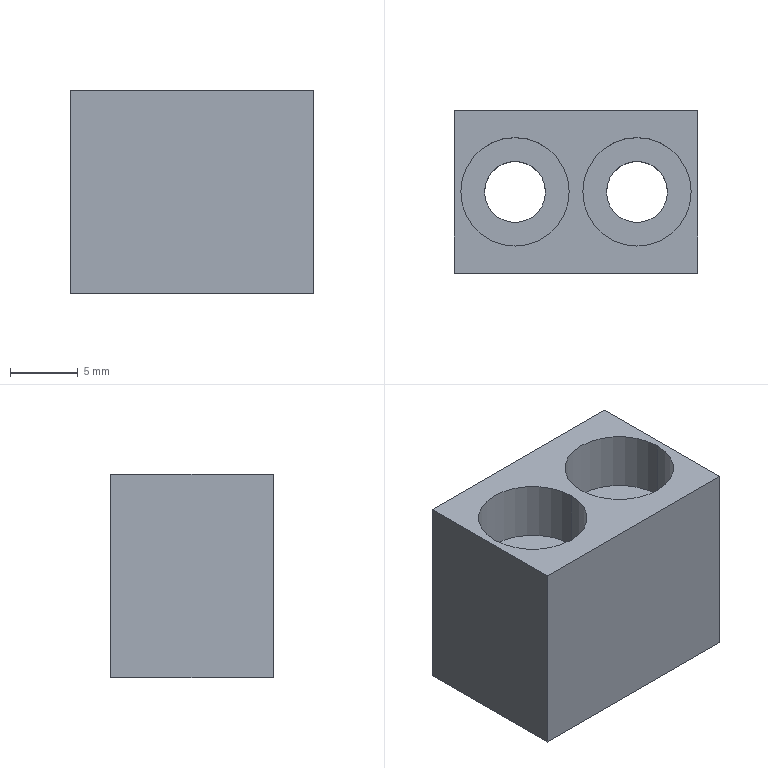Part | SolidWorks | features BaseBody 1 | 1 solid | 16 faces | box 18 x 12 x 15 mm | volume 2460 mm3 | cylinder 8 | plane 8 | commonest cylinder face diameters 4.5 x4 8 x4
STEP:
#1=CARTESIAN_POINT('',(-2.25,0.,0.));
#2=VERTEX_POINT('',#1);
#3=CARTESIAN_POINT('',(-6.75,0.,0.));
#4=VERTEX_POINT('',#3);
#5=CARTESIAN_POINT('',(-4.5,0.,0.));
#6=DIRECTION('',(0.,0.,-1.));
#7=DIRECTION('',(1.,0.,0.));
#8=AXIS2_PLACEMENT_3D('',#5,#6,#7);
#9=CIRCLE('',#8,2.25);
#10=EDGE_CURVE('',#2,#4,#9,.T.);
#11=ORIENTED_EDGE('',*,*,#10,.T.);
#12=CARTESIAN_POINT('',(-6.75,0.,10.6));
#13=VERTEX_POINT('',#12);
#14=CARTESIAN_POINT('',(-6.75,0.,15.));
#15=DIRECTION('',(0.,0.,1.));
#16=VECTOR('',#15,1000.);
#17=LINE('',#14,#16);
#18=EDGE_CURVE('',#4,#13,#17,.T.);
#19=ORIENTED_EDGE('',*,*,#18,.T.);
#20=CARTESIAN_POINT('',(-2.25,0.,10.6));
#21=VERTEX_POINT('',#20);
#22=CARTESIAN_POINT('',(-4.5,0.,10.6));
#23=DIRECTION('',(0.,0.,-1.));
#24=DIRECTION('',(1.,0.,0.));
#25=AXIS2_PLACEMENT_3D('',#22,#23,#24);
#26=CIRCLE('',#25,2.25);
#27=EDGE_CURVE('',#21,#13,#26,.T.);
#28=ORIENTED_EDGE('',*,*,#27,.F.);
#29=CARTESIAN_POINT('',(-2.25,0.,15.));
#30=DIRECTION('',(0.,0.,1.));
#31=VECTOR('',#30,1000.);
#32=LINE('',#29,#31);
#33=EDGE_CURVE('',#2,#21,#32,.T.);
#34=ORIENTED_EDGE('',*,*,#33,.F.);
#35=EDGE_LOOP('',(#11,#19,#28,#34));
#36=FACE_OUTER_BOUND('',#35,.T.);
#37=CARTESIAN_POINT('',(-4.5,0.,15.));
#38=DIRECTION('',(0.,0.,1.));
#39=DIRECTION('',(1.,0.,0.));
#40=AXIS2_PLACEMENT_3D('',#37,#38,#39);
#41=CYLINDRICAL_SURFACE('',#40,2.25);
#42=ADVANCED_FACE('',(#36),#41,.F.);
#43=CARTESIAN_POINT('',(6.75,0.,0.));
#44=VERTEX_POINT('',#43);
#45=CARTESIAN_POINT('',(2.25,0.,0.));
#46=VERTEX_POINT('',#45);
#47=CARTESIAN_POINT('',(4.5,0.,0.));
#48=DIRECTION('',(0.,0.,-1.));
#49=DIRECTION('',(1.,0.,0.));
#50=AXIS2_PLACEMENT_3D('',#47,#48,#49);
#51=CIRCLE('',#50,2.25);
#52=EDGE_CURVE('',#44,#46,#51,.T.);
#53=ORIENTED_EDGE('',*,*,#52,.T.);
#54=CARTESIAN_POINT('',(2.25,0.,10.6));
#55=VERTEX_POINT('',#54);
#56=CARTESIAN_POINT('',(2.25,0.,15.));
#57=DIRECTION('',(0.,0.,1.));
#58=VECTOR('',#57,1000.);
#59=LINE('',#56,#58);
#60=EDGE_CURVE('',#46,#55,#59,.T.);
#61=ORIENTED_EDGE('',*,*,#60,.T.);
#62=CARTESIAN_POINT('',(6.75,0.,10.6));
#63=VERTEX_POINT('',#62);
#64=CARTESIAN_POINT('',(4.5,0.,10.6));
#65=DIRECTION('',(0.,0.,-1.));
#66=DIRECTION('',(1.,0.,0.));
#67=AXIS2_PLACEMENT_3D('',#64,#65,#66);
#68=CIRCLE('',#67,2.25);
#69=EDGE_CURVE('',#63,#55,#68,.T.);
#70=ORIENTED_EDGE('',*,*,#69,.F.);
#71=CARTESIAN_POINT('',(6.75,0.,15.));
#72=DIRECTION('',(0.,0.,1.));
#73=VECTOR('',#72,1000.);
#74=LINE('',#71,#73);
#75=EDGE_CURVE('',#44,#63,#74,.T.);
#76=ORIENTED_EDGE('',*,*,#75,.F.);
#77=EDGE_LOOP('',(#53,#61,#70,#76));
#78=FACE_OUTER_BOUND('',#77,.T.);
#79=CARTESIAN_POINT('',(4.5,0.,15.));
#80=DIRECTION('',(0.,0.,1.));
#81=DIRECTION('',(1.,0.,0.));
#82=AXIS2_PLACEMENT_3D('',#79,#80,#81);
#83=CYLINDRICAL_SURFACE('',#82,2.25);
#84=ADVANCED_FACE('',(#78),#83,.F.);
#85=CARTESIAN_POINT('',(-8.5,0.,10.6));
#86=VERTEX_POINT('',#85);
#87=CARTESIAN_POINT('',(-0.5,0.,10.6));
#88=VERTEX_POINT('',#87);
#89=CARTESIAN_POINT('',(-4.5,0.,10.6));
#90=DIRECTION('',(0.,0.,1.));
#91=DIRECTION('',(1.,0.,0.));
#92=AXIS2_PLACEMENT_3D('',#89,#90,#91);
#93=CIRCLE('',#92,4.);
#94=EDGE_CURVE('',#86,#88,#93,.T.);
#95=ORIENTED_EDGE('',*,*,#94,.F.);
#96=CARTESIAN_POINT('',(-8.5,0.,15.));
#97=VERTEX_POINT('',#96);
#98=CARTESIAN_POINT('',(-8.5,0.,15.));
#99=DIRECTION('',(0.,0.,1.));
#100=VECTOR('',#99,1000.);
#101=LINE('',#98,#100);
#102=EDGE_CURVE('',#86,#97,#101,.T.);
#103=ORIENTED_EDGE('',*,*,#102,.T.);
#104=CARTESIAN_POINT('',(-0.5,0.,15.));
#105=VERTEX_POINT('',#104);
#106=CARTESIAN_POINT('',(-4.5,0.,15.));
#107=DIRECTION('',(0.,0.,-1.));
#108=DIRECTION('',(1.,0.,0.));
#109=AXIS2_PLACEMENT_3D('',#106,#107,#108);
#110=CIRCLE('',#109,4.);
#111=EDGE_CURVE('',#105,#97,#110,.T.);
#112=ORIENTED_EDGE('',*,*,#111,.F.);
#113=CARTESIAN_POINT('',(-0.5,0.,15.));
#114=DIRECTION('',(0.,0.,1.));
#115=VECTOR('',#114,1000.);
#116=LINE('',#113,#115);
#117=EDGE_CURVE('',#88,#105,#116,.T.);
#118=ORIENTED_EDGE('',*,*,#117,.F.);
#119=EDGE_LOOP('',(#95,#103,#112,#118));
#120=FACE_OUTER_BOUND('',#119,.T.);
#121=CARTESIAN_POINT('',(-4.5,0.,15.));
#122=DIRECTION('',(0.,0.,1.));
#123=DIRECTION('',(1.,0.,0.));
#124=AXIS2_PLACEMENT_3D('',#121,#122,#123);
#125=CYLINDRICAL_SURFACE('',#124,4.);
#126=ADVANCED_FACE('',(#120),#125,.F.);
#127=CARTESIAN_POINT('',(0.5,0.,10.6));
#128=VERTEX_POINT('',#127);
#129=CARTESIAN_POINT('',(8.5,0.,10.6));
#130=VERTEX_POINT('',#129);
#131=CARTESIAN_POINT('',(4.5,0.,10.6));
#132=DIRECTION('',(0.,0.,1.));
#133=DIRECTION('',(1.,0.,0.));
#134=AXIS2_PLACEMENT_3D('',#131,#132,#133);
#135=CIRCLE('',#134,4.);
#136=EDGE_CURVE('',#128,#130,#135,.T.);
#137=ORIENTED_EDGE('',*,*,#136,.F.);
#138=CARTESIAN_POINT('',(0.5,0.,15.));
#139=VERTEX_POINT('',#138);
#140=CARTESIAN_POINT('',(0.5,0.,15.));
#141=DIRECTION('',(0.,0.,1.));
#142=VECTOR('',#141,1000.);
#143=LINE('',#140,#142);
#144=EDGE_CURVE('',#128,#139,#143,.T.);
#145=ORIENTED_EDGE('',*,*,#144,.T.);
#146=CARTESIAN_POINT('',(8.5,0.,15.));
#147=VERTEX_POINT('',#146);
#148=CARTESIAN_POINT('',(4.5,0.,15.));
#149=DIRECTION('',(0.,0.,-1.));
#150=DIRECTION('',(1.,0.,0.));
#151=AXIS2_PLACEMENT_3D('',#148,#149,#150);
#152=CIRCLE('',#151,4.);
#153=EDGE_CURVE('',#147,#139,#152,.T.);
#154=ORIENTED_EDGE('',*,*,#153,.F.);
#155=CARTESIAN_POINT('',(8.5,0.,15.));
#156=DIRECTION('',(0.,0.,1.));
#157=VECTOR('',#156,1000.);
#158=LINE('',#155,#157);
#159=EDGE_CURVE('',#130,#147,#158,.T.);
#160=ORIENTED_EDGE('',*,*,#159,.F.);
#161=EDGE_LOOP('',(#137,#145,#154,#160));
#162=FACE_OUTER_BOUND('',#161,.T.);
#163=CARTESIAN_POINT('',(4.5,0.,15.));
#164=DIRECTION('',(0.,0.,1.));
#165=DIRECTION('',(1.,0.,0.));
#166=AXIS2_PLACEMENT_3D('',#163,#164,#165);
#167=CYLINDRICAL_SURFACE('',#166,4.);
#168=ADVANCED_FACE('',(#162),#167,.F.);
#169=CARTESIAN_POINT('',(-9.,6.,15.));
#170=VERTEX_POINT('',#169);
#171=CARTESIAN_POINT('',(-9.,6.,0.));
#172=VERTEX_POINT('',#171);
#173=CARTESIAN_POINT('',(-9.,6.,15.));
#174=DIRECTION('',(0.,0.,-1.));
#175=VECTOR('',#174,1000.);
#176=LINE('',#173,#175);
#177=EDGE_CURVE('',#170,#172,#176,.T.);
#178=ORIENTED_EDGE('',*,*,#177,.F.);
#179=CARTESIAN_POINT('',(9.,6.,15.));
#180=VERTEX_POINT('',#179);
#181=CARTESIAN_POINT('',(-9.,6.,15.));
#182=DIRECTION('',(-1.,0.,0.));
#183=VECTOR('',#182,1000.);
#184=LINE('',#181,#183);
#185=EDGE_CURVE('',#180,#170,#184,.T.);
#186=ORIENTED_EDGE('',*,*,#185,.F.);
#187=CARTESIAN_POINT('',(9.,6.,0.));
#188=VERTEX_POINT('',#187);
#189=CARTESIAN_POINT('',(9.,6.,15.));
#190=DIRECTION('',(0.,0.,1.));
#191=VECTOR('',#190,1000.);
#192=LINE('',#189,#191);
#193=EDGE_CURVE('',#188,#180,#192,.T.);
#194=ORIENTED_EDGE('',*,*,#193,.F.);
#195=CARTESIAN_POINT('',(-9.,6.,0.));
#196=DIRECTION('',(1.,0.,0.));
#197=VECTOR('',#196,1000.);
#198=LINE('',#195,#197);
#199=EDGE_CURVE('',#172,#188,#198,.T.);
#200=ORIENTED_EDGE('',*,*,#199,.F.);
#201=EDGE_LOOP('',(#178,#186,#194,#200));
#202=FACE_OUTER_BOUND('',#201,.T.);
#203=CARTESIAN_POINT('',(-9.,6.,15.));
#204=DIRECTION('',(0.,-1.,0.));
#205=DIRECTION('',(0.,0.,-1.));
#206=AXIS2_PLACEMENT_3D('',#203,#204,#205);
#207=PLANE('',#206);
#208=ADVANCED_FACE('',(#202),#207,.F.);
#209=CARTESIAN_POINT('',(-9.,-6.,0.));
#210=VERTEX_POINT('',#209);
#211=CARTESIAN_POINT('',(9.,-6.,0.));
#212=VERTEX_POINT('',#211);
#213=CARTESIAN_POINT('',(0.,-6.,0.));
#214=DIRECTION('',(1.,0.,0.));
#215=VECTOR('',#214,1000.);
#216=LINE('',#213,#215);
#217=EDGE_CURVE('',#210,#212,#216,.T.);
#218=ORIENTED_EDGE('',*,*,#217,.F.);
#219=CARTESIAN_POINT('',(-9.,0.,0.));
#220=DIRECTION('',(0.,-1.,0.));
#221=VECTOR('',#220,1000.);
#222=LINE('',#219,#221);
#223=EDGE_CURVE('',#172,#210,#222,.T.);
#224=ORIENTED_EDGE('',*,*,#223,.F.);
#225=ORIENTED_EDGE('',*,*,#199,.T.);
#226=CARTESIAN_POINT('',(9.,0.,0.));
#227=DIRECTION('',(0.,1.,0.));
#228=VECTOR('',#227,1000.);
#229=LINE('',#226,#228);
#230=EDGE_CURVE('',#212,#188,#229,.T.);
#231=ORIENTED_EDGE('',*,*,#230,.F.);
#232=EDGE_LOOP('',(#218,#224,#225,#231));
#233=FACE_OUTER_BOUND('',#232,.T.);
#234=ORIENTED_EDGE('',*,*,#10,.F.);
#235=CARTESIAN_POINT('',(-4.5,0.,0.));
#236=DIRECTION('',(0.,0.,-1.));
#237=DIRECTION('',(1.,0.,0.));
#238=AXIS2_PLACEMENT_3D('',#235,#236,#237);
#239=CIRCLE('',#238,2.25);
#240=EDGE_CURVE('',#4,#2,#239,.T.);
#241=ORIENTED_EDGE('',*,*,#240,.F.);
#242=EDGE_LOOP('',(#234,#241));
#243=FACE_BOUND('',#242,.T.);
#244=ORIENTED_EDGE('',*,*,#52,.F.);
#245=CARTESIAN_POINT('',(4.5,0.,0.));
#246=DIRECTION('',(0.,0.,-1.));
#247=DIRECTION('',(1.,0.,0.));
#248=AXIS2_PLACEMENT_3D('',#245,#246,#247);
#249=CIRCLE('',#248,2.25);
#250=EDGE_CURVE('',#46,#44,#249,.T.);
#251=ORIENTED_EDGE('',*,*,#250,.F.);
#252=EDGE_LOOP('',(#244,#251));
#253=FACE_BOUND('',#252,.T.);
#254=CARTESIAN_POINT('',(0.,0.,0.));
#255=DIRECTION('',(0.,0.,1.));
#256=DIRECTION('',(1.,0.,0.));
#257=AXIS2_PLACEMENT_3D('',#254,#255,#256);
#258=PLANE('',#257);
#259=ADVANCED_FACE('',(#233,#243,#253),#258,.F.);
#260=CARTESIAN_POINT('',(-9.,-6.,15.));
#261=VERTEX_POINT('',#260);
#262=CARTESIAN_POINT('',(-9.,-6.,15.));
#263=DIRECTION('',(0.,0.,-1.));
#264=VECTOR('',#263,1000.);
#265=LINE('',#262,#264);
#266=EDGE_CURVE('',#261,#210,#265,.T.);
#267=ORIENTED_EDGE('',*,*,#266,.F.);
#268=CARTESIAN_POINT('',(-9.,6.,15.));
#269=DIRECTION('',(0.,-1.,0.));
#270=VECTOR('',#269,1000.);
#271=LINE('',#268,#270);
#272=EDGE_CURVE('',#170,#261,#271,.T.);
#273=ORIENTED_EDGE('',*,*,#272,.F.);
#274=ORIENTED_EDGE('',*,*,#177,.T.);
#275=ORIENTED_EDGE('',*,*,#223,.T.);
#276=EDGE_LOOP('',(#267,#273,#274,#275));
#277=FACE_OUTER_BOUND('',#276,.T.);
#278=CARTESIAN_POINT('',(-9.,6.,15.));
#279=DIRECTION('',(1.,0.,0.));
#280=DIRECTION('',(0.,0.,-1.));
#281=AXIS2_PLACEMENT_3D('',#278,#279,#280);
#282=PLANE('',#281);
#283=ADVANCED_FACE('',(#277),#282,.F.);
#284=ORIENTED_EDGE('',*,*,#272,.T.);
#285=CARTESIAN_POINT('',(9.,-6.,15.));
#286=VERTEX_POINT('',#285);
#287=CARTESIAN_POINT('',(0.,-6.,15.));
#288=DIRECTION('',(1.,0.,0.));
#289=VECTOR('',#288,1000.);
#290=LINE('',#287,#289);
#291=EDGE_CURVE('',#261,#286,#290,.T.);
#292=ORIENTED_EDGE('',*,*,#291,.T.);
#293=CARTESIAN_POINT('',(9.,0.,15.));
#294=DIRECTION('',(0.,1.,0.));
#295=VECTOR('',#294,1000.);
#296=LINE('',#293,#295);
#297=EDGE_CURVE('',#286,#180,#296,.T.);
#298=ORIENTED_EDGE('',*,*,#297,.T.);
#299=ORIENTED_EDGE('',*,*,#185,.T.);
#300=EDGE_LOOP('',(#284,#292,#298,#299));
#301=FACE_OUTER_BOUND('',#300,.T.);
#302=ORIENTED_EDGE('',*,*,#111,.T.);
#303=CARTESIAN_POINT('',(-4.5,0.,15.));
#304=DIRECTION('',(0.,0.,-1.));
#305=DIRECTION('',(1.,0.,0.));
#306=AXIS2_PLACEMENT_3D('',#303,#304,#305);
#307=CIRCLE('',#306,4.);
#308=EDGE_CURVE('',#97,#105,#307,.T.);
#309=ORIENTED_EDGE('',*,*,#308,.T.);
#310=EDGE_LOOP('',(#302,#309));
#311=FACE_BOUND('',#310,.T.);
#312=ORIENTED_EDGE('',*,*,#153,.T.);
#313=CARTESIAN_POINT('',(4.5,0.,15.));
#314=DIRECTION('',(0.,0.,-1.));
#315=DIRECTION('',(1.,0.,0.));
#316=AXIS2_PLACEMENT_3D('',#313,#314,#315);
#317=CIRCLE('',#316,4.);
#318=EDGE_CURVE('',#139,#147,#317,.T.);
#319=ORIENTED_EDGE('',*,*,#318,.T.);
#320=EDGE_LOOP('',(#312,#319));
#321=FACE_BOUND('',#320,.T.);
#322=CARTESIAN_POINT('',(0.,0.,15.));
#323=DIRECTION('',(0.,0.,1.));
#324=DIRECTION('',(1.,0.,0.));
#325=AXIS2_PLACEMENT_3D('',#322,#323,#324);
#326=PLANE('',#325);
#327=ADVANCED_FACE('',(#301,#311,#321),#326,.T.);
#328=ORIENTED_EDGE('',*,*,#193,.T.);
#329=ORIENTED_EDGE('',*,*,#297,.F.);
#330=CARTESIAN_POINT('',(9.,-6.,15.));
#331=DIRECTION('',(0.,0.,1.));
#332=VECTOR('',#331,1000.);
#333=LINE('',#330,#332);
#334=EDGE_CURVE('',#212,#286,#333,.T.);
#335=ORIENTED_EDGE('',*,*,#334,.F.);
#336=ORIENTED_EDGE('',*,*,#230,.T.);
#337=EDGE_LOOP('',(#328,#329,#335,#336));
#338=FACE_OUTER_BOUND('',#337,.T.);
#339=CARTESIAN_POINT('',(9.,6.,15.));
#340=DIRECTION('',(-1.,0.,0.));
#341=DIRECTION('',(0.,-1.,0.));
#342=AXIS2_PLACEMENT_3D('',#339,#340,#341);
#343=PLANE('',#342);
#344=ADVANCED_FACE('',(#338),#343,.F.);
#345=ORIENTED_EDGE('',*,*,#334,.T.);
#346=ORIENTED_EDGE('',*,*,#291,.F.);
#347=ORIENTED_EDGE('',*,*,#266,.T.);
#348=ORIENTED_EDGE('',*,*,#217,.T.);
#349=EDGE_LOOP('',(#345,#346,#347,#348));
#350=FACE_OUTER_BOUND('',#349,.T.);
#351=CARTESIAN_POINT('',(-9.,-6.,15.));
#352=DIRECTION('',(0.,1.,0.));
#353=DIRECTION('',(0.,0.,1.));
#354=AXIS2_PLACEMENT_3D('',#351,#352,#353);
#355=PLANE('',#354);
#356=ADVANCED_FACE('',(#350),#355,.F.);
#357=ORIENTED_EDGE('',*,*,#18,.F.);
#358=ORIENTED_EDGE('',*,*,#240,.T.);
#359=ORIENTED_EDGE('',*,*,#33,.T.);
#360=CARTESIAN_POINT('',(-4.5,0.,10.6));
#361=DIRECTION('',(0.,0.,-1.));
#362=DIRECTION('',(1.,0.,0.));
#363=AXIS2_PLACEMENT_3D('',#360,#361,#362);
#364=CIRCLE('',#363,2.25);
#365=EDGE_CURVE('',#13,#21,#364,.T.);
#366=ORIENTED_EDGE('',*,*,#365,.F.);
#367=EDGE_LOOP('',(#357,#358,#359,#366));
#368=FACE_OUTER_BOUND('',#367,.T.);
#369=CARTESIAN_POINT('',(-4.5,0.,15.));
#370=DIRECTION('',(0.,0.,1.));
#371=DIRECTION('',(1.,0.,0.));
#372=AXIS2_PLACEMENT_3D('',#369,#370,#371);
#373=CYLINDRICAL_SURFACE('',#372,2.25);
#374=ADVANCED_FACE('',(#368),#373,.F.);
#375=ORIENTED_EDGE('',*,*,#60,.F.);
#376=ORIENTED_EDGE('',*,*,#250,.T.);
#377=ORIENTED_EDGE('',*,*,#75,.T.);
#378=CARTESIAN_POINT('',(4.5,0.,10.6));
#379=DIRECTION('',(0.,0.,-1.));
#380=DIRECTION('',(1.,0.,0.));
#381=AXIS2_PLACEMENT_3D('',#378,#379,#380);
#382=CIRCLE('',#381,2.25);
#383=EDGE_CURVE('',#55,#63,#382,.T.);
#384=ORIENTED_EDGE('',*,*,#383,.F.);
#385=EDGE_LOOP('',(#375,#376,#377,#384));
#386=FACE_OUTER_BOUND('',#385,.T.);
#387=CARTESIAN_POINT('',(4.5,0.,15.));
#388=DIRECTION('',(0.,0.,1.));
#389=DIRECTION('',(1.,0.,0.));
#390=AXIS2_PLACEMENT_3D('',#387,#388,#389);
#391=CYLINDRICAL_SURFACE('',#390,2.25);
#392=ADVANCED_FACE('',(#386),#391,.F.);
#393=ORIENTED_EDGE('',*,*,#102,.F.);
#394=CARTESIAN_POINT('',(-4.5,0.,10.6));
#395=DIRECTION('',(0.,0.,1.));
#396=DIRECTION('',(1.,0.,0.));
#397=AXIS2_PLACEMENT_3D('',#394,#395,#396);
#398=CIRCLE('',#397,4.);
#399=EDGE_CURVE('',#88,#86,#398,.T.);
#400=ORIENTED_EDGE('',*,*,#399,.F.);
#401=ORIENTED_EDGE('',*,*,#117,.T.);
#402=ORIENTED_EDGE('',*,*,#308,.F.);
#403=EDGE_LOOP('',(#393,#400,#401,#402));
#404=FACE_OUTER_BOUND('',#403,.T.);
#405=CARTESIAN_POINT('',(-4.5,0.,15.));
#406=DIRECTION('',(0.,0.,1.));
#407=DIRECTION('',(1.,0.,0.));
#408=AXIS2_PLACEMENT_3D('',#405,#406,#407);
#409=CYLINDRICAL_SURFACE('',#408,4.);
#410=ADVANCED_FACE('',(#404),#409,.F.);
#411=ORIENTED_EDGE('',*,*,#144,.F.);
#412=CARTESIAN_POINT('',(4.5,0.,10.6));
#413=DIRECTION('',(0.,0.,1.));
#414=DIRECTION('',(1.,0.,0.));
#415=AXIS2_PLACEMENT_3D('',#412,#413,#414);
#416=CIRCLE('',#415,4.);
#417=EDGE_CURVE('',#130,#128,#416,.T.);
#418=ORIENTED_EDGE('',*,*,#417,.F.);
#419=ORIENTED_EDGE('',*,*,#159,.T.);
#420=ORIENTED_EDGE('',*,*,#318,.F.);
#421=EDGE_LOOP('',(#411,#418,#419,#420));
#422=FACE_OUTER_BOUND('',#421,.T.);
#423=CARTESIAN_POINT('',(4.5,0.,15.));
#424=DIRECTION('',(0.,0.,1.));
#425=DIRECTION('',(1.,0.,0.));
#426=AXIS2_PLACEMENT_3D('',#423,#424,#425);
#427=CYLINDRICAL_SURFACE('',#426,4.);
#428=ADVANCED_FACE('',(#422),#427,.F.);
#429=ORIENTED_EDGE('',*,*,#399,.T.);
#430=ORIENTED_EDGE('',*,*,#94,.T.);
#431=EDGE_LOOP('',(#429,#430));
#432=FACE_OUTER_BOUND('',#431,.T.);
#433=ORIENTED_EDGE('',*,*,#27,.T.);
#434=ORIENTED_EDGE('',*,*,#365,.T.);
#435=EDGE_LOOP('',(#433,#434));
#436=FACE_BOUND('',#435,.T.);
#437=CARTESIAN_POINT('',(-2.25,0.,10.6));
#438=DIRECTION('',(0.,0.,-1.));
#439=DIRECTION('',(-1.,0.,0.));
#440=AXIS2_PLACEMENT_3D('',#437,#438,#439);
#441=PLANE('',#440);
#442=ADVANCED_FACE('',(#432,#436),#441,.F.);
#443=ORIENTED_EDGE('',*,*,#417,.T.);
#444=ORIENTED_EDGE('',*,*,#136,.T.);
#445=EDGE_LOOP('',(#443,#444));
#446=FACE_OUTER_BOUND('',#445,.T.);
#447=ORIENTED_EDGE('',*,*,#69,.T.);
#448=ORIENTED_EDGE('',*,*,#383,.T.);
#449=EDGE_LOOP('',(#447,#448));
#450=FACE_BOUND('',#449,.T.);
#451=CARTESIAN_POINT('',(6.75,0.,10.6));
#452=DIRECTION('',(0.,0.,-1.));
#453=DIRECTION('',(-1.,0.,0.));
#454=AXIS2_PLACEMENT_3D('',#451,#452,#453);
#455=PLANE('',#454);
#456=ADVANCED_FACE('',(#446,#450),#455,.F.);
#457=CLOSED_SHELL('',(#42,#84,#126,#168,#208,#259,#283,#327,#344,#356,#374,#392,#410,#428,#442,#456));
#458=MANIFOLD_SOLID_BREP('',#457);
#459=CARTESIAN_POINT('',(0.,0.,0.));
#460=DIRECTION('',(0.,0.,1.));
#461=DIRECTION('',(1.,0.,0.));
#462=AXIS2_PLACEMENT_3D('',#459,#460,#461);
#463=(LENGTH_UNIT()NAMED_UNIT(*)SI_UNIT(.MILLI.,.METRE.));
#464=UNCERTAINTY_MEASURE_WITH_UNIT(LENGTH_MEASURE(0.00001),#463,'','');
#465=(NAMED_UNIT(*)PLANE_ANGLE_UNIT()SI_UNIT($,.RADIAN.));
#466=(NAMED_UNIT(*)SI_UNIT($,.STERADIAN.)SOLID_ANGLE_UNIT());
#467=(GEOMETRIC_REPRESENTATION_CONTEXT(3)GLOBAL_UNCERTAINTY_ASSIGNED_CONTEXT((#464))GLOBAL_UNIT_ASSIGNED_CONTEXT((#463,#465,#466))REPRESENTATION_CONTEXT('',''));
#468=ADVANCED_BREP_SHAPE_REPRESENTATION('',(#458,#462),#467);